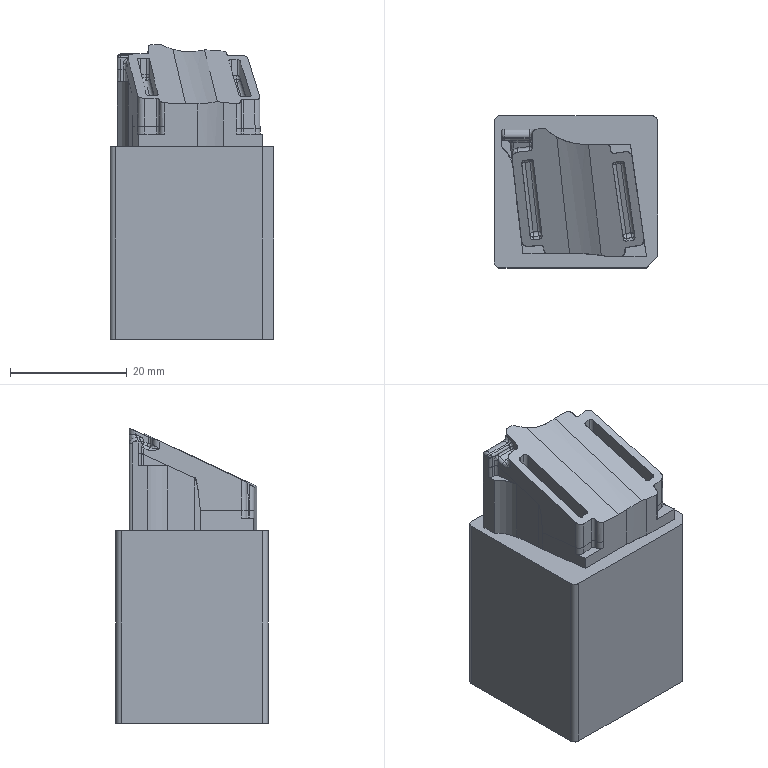NC program | NX | posted with a generic post | part box 28 x 26 x 50.455 mm
Whole program:
N10 G17 G21 G94 G90
(CAVITY_MILL_COPY_COPY_COPY , TOOL : D6)
N12 T00 M6
N14 G54
N16 G17 G0 G90 X-16.065 Y-6.944 S0 M3
N18 G43 Z10. H0
N20 Z-17.155
N22 G94 G1 Z-17.455 F250.
N24 G3 X-13.444 Y-3.607 R3.
N26 G1 X-13.656 Y-1.849
N28 G2 X-13.68 Y-1.506 R3.5
N30 G3 X-13.722 Y-0.893 R6.5
N32 G1 X-14.267 Y3.803
N34 G3 X-14.887 Y4.891 R1.6
N36 G2 X-16.265 Y7.674 R3.5
N38 G1 Y10.218
N40 G2 X-12.265 Y14.218 R4.
N42 G1 X-5.218
N44 G2 X-2.85 Y13.295 R3.5
N46 G3 X1.548 Y11.581 R6.5
N48 G1 X9.331
N50 G2 X12.793 Y8.593 R3.5
N52 G1 X12.81 Y8.596
N54 X12.815 Y8.555
N56 X12.799 Y8.553
N58 X15.516 Y-10.582
N60 G2 X12.05 Y-14.574 R3.5
N62 G1 X5.364
N64 G2 X4.602 Y-14.49 R3.5
N66 G3 X1.011 Y-14.094 R16.5
N68 G1 X-9.08
N70 G2 X-12.555 Y-11.012 R3.5
N72 G1 X-13.444 Y-3.607
N74 G3 X-16.781 Y-0.987 R3.
N76 G1 Z-17.155
N78 G0 Z10.
N80 M5
N82 M2